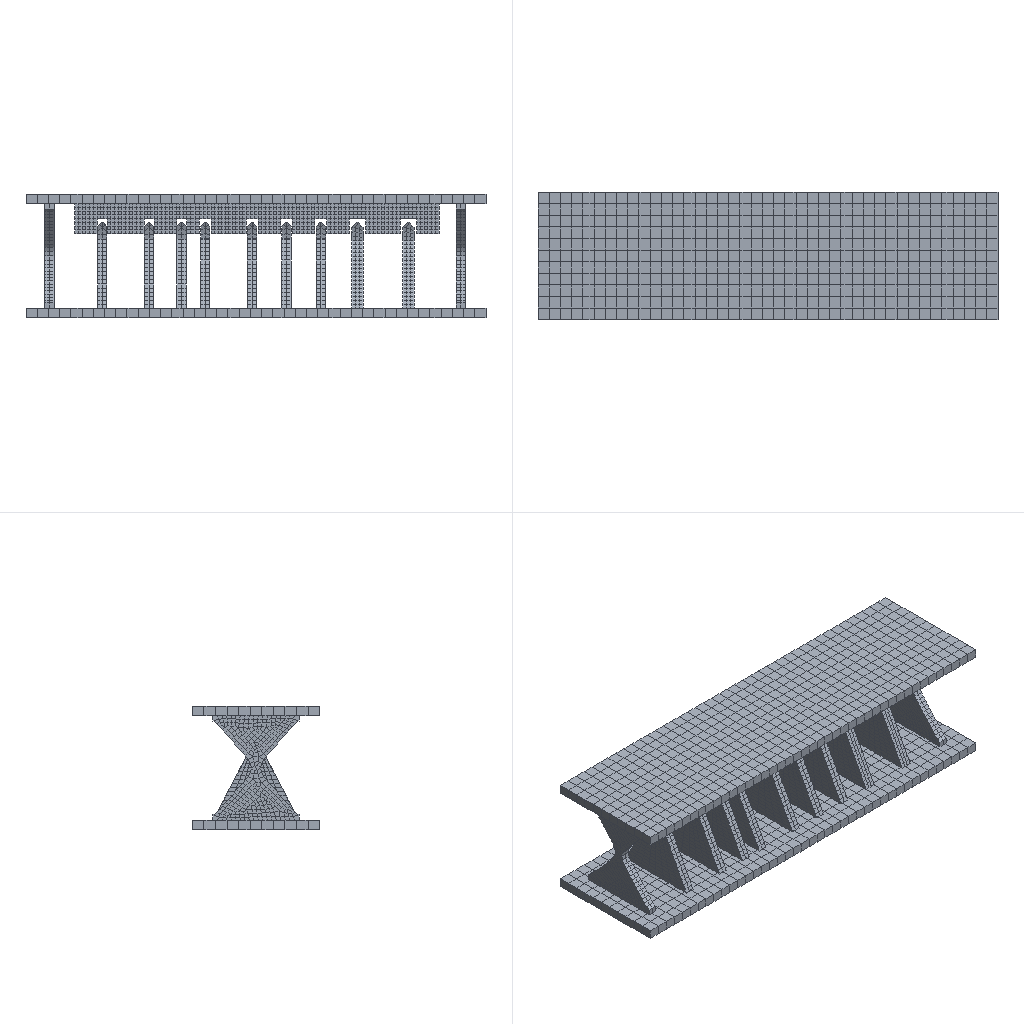Simulation study | abaqus
Abaqus input file, long lists of numbers shortened:
*Heading
** Job name: deck-2 Model name: 0815
** Generated by: Abaqus/CAE 2024
*Preprint, echo=NO, model=NO, history=NO, contact=NO
**
** PARTS
**
*Part, name=Part-1
*Node
      1,      1227.62,         340.,          25.
      2,      1227.62,   309.091,          25.
** (1006 more lines like these left out)
*Element, type=C3D8R
  1,   25,   26,   38,   37,    1,    2,   14,   13
  2,   26,   27,   39,   38,    2,    3,   15,   14
** (449 more lines like these left out)
*Nset, nset=_PickedSet5, internal, generate
    1,  1008,     1
*Elset, elset=_PickedSet5, internal, generate
   1,  451,    1
** Section: q235
*Solid Section, elset=_PickedSet5, controls=EC-1, material=q235
,
*End Part
**
*Part, name=Part-7
*Node
      1,   51318.848,   20056.129,           0.
      2,      51308.5,   20050.193,           0.
** (1084 more lines like these left out)
*Element, type=C3D8R
  1,  119,    1,    2,  145,  481,  363,  364,  507
  2,    1,  119,  116,   23,  363,  481,  478,  385
** (622 more lines like these left out)
*Nset, nset=Set-1, generate
    1,  1086,     1
*Elset, elset=Set-1, generate
   1,  624,    1
** Section: Section-2
*Solid Section, elset=Set-1, material=q235
,
*End Part
**
*Part, name=Part-8
*Node
      1,   44.972,         218.,           0.
      2,   50.449,         230.,          10.
** (601 more lines like these left out)
*Element, type=C3D8R
 1, 164,  20, 157, 481,  18,   1,  19, 155
 2, 165,  21, 158, 480, 164,  20, 157, 481
** (334 more lines like these left out)
*Nset, nset=Set-1, generate
   1,  603,    1
*Elset, elset=Set-1, generate
   1,  336,    1
** Section: Section-2
*Solid Section, elset=Set-1, material=q235
,
*End Part
**
*Part, name=Part-9
*Node
      1,  -916.483,   84.154,           0.
      2,  -916.483,   84.154,          40.
** (4008 more lines like these left out)
*Element, type=C3D8R
 1,  158, 1029, 2787,  999,    1,  121,  969,  136
 2, 1029, 1030, 2788, 2787,  121,  122,  970,  969
** (2638 more lines like these left out)
*Nset, nset=Set-1, generate
    1,  4010,     1
*Elset, elset=Set-1, generate
    1,  2640,     1
** Section: Section-2
*Solid Section, elset=Set-1, material=q235
,
*End Part
**
*Part, name=Part-10
*Node
      1,   4.129,   256.243,          25.
      2,   4.785,   252.357,          25.
** (558 more lines like these left out)
*Element, type=C3D8R
 1,  36,  43, 171, 165,   1,   2,  21,  22
 2, 165, 171,  42,  25,  22,  21,   3,   4
** (306 more lines like these left out)
*Nset, nset=Set-1
   1,   2,   3,   4,   5,   6,   7,   8,  17,  18,  19,  20,  21,  22,  23,  24
  25,  26,  27,  28,  29,  30,  31,  32,  33,  34,  35,  36,  37,  38,  39,  40
** (27 more lines like these left out)
*Elset, elset=Set-1
   1,   2,   3,   4,   5,   6,   7,   8,   9,  10,  11,  12,  13,  14,  71,  72
  73,  74,  75,  76,  77,  78,  79,  80,  81,  82,  83,  84,  85,  86,  87,  88
** (14 more lines like these left out)
*Nset, nset=_PickedSet10, internal, generate
   1,  560,    1
*Elset, elset=_PickedSet10, internal, generate
   1,  308,    1
** Section: Section-2
*Solid Section, elset=_PickedSet10, material=q235
,
*End Part
**
*Part, name=Part-11
*Node
      1,  -175.665,   409.503,         17.5
      2,  -105.665,   409.503,         17.5
** (878 more lines like these left out)
*Element, type=C3D8R
  1,   4,  22,   7,   1,  44,  62,  47,  41
  2,  22,  21,   8,   7,  62,  61,  48,  47
** (565 more lines like these left out)
*Nset, nset=Set-1, generate
   1,  880,    1
*Elset, elset=Set-1, generate
   1,  567,    1
** Section: Section-2
*Solid Section, elset=Set-1, material=q235
,
*End Part
**
**
** ASSEMBLY
**
*Assembly, name=Assembly
**
*Instance, name=Part-1-1, part=Part-1
*End Instance
**
*Instance, name=Part-1-1-lin-2-1, part=Part-1
          0.,           0.,         305.
*End Instance
**
*Instance, name=Part-7-1, part=Part-7
50.,     -51253.5, -20010.046
50.,     -51253.5, -20010.046, 50.577, -51252.923, -20009.469,         120.
*End Instance
**
*Instance, name=Part-7-1-lin-2-1, part=Part-7
     1147.62,     -51253.5, -20010.046
     1147.62,     -51253.5, -20010.046, 1148.197, -51252.923, -20009.469,         120.
*End Instance
**
*Instance, name=Part-9-1, part=Part-9
 1106.483,         190.,   180.846
 1106.483,         190.,   180.846, 1107.483,         190.,   180.846, 90.
*End Instance
**
*Instance, name=Part-8-1, part=Part-8
      190.85,   152.051,          25.
      190.85,   152.051,          25., 191.427, 152.628, 25.577,         120.
*End Instance
**
*Instance, name=Part-8-1-lin-1-2, part=Part-8
      315.85,   152.051,          25.
      315.85,   152.051,          25., 316.427, 152.628, 25.577,         120.
*End Instance
**
*Instance, name=Part-8-1-lin-1-2-lin-2-1, part=Part-8
      402.55,   152.051,          25.
      402.55,   152.051,          25., 403.127, 152.628, 25.577,         120.
*End Instance
**
*Instance, name=Part-10-1, part=Part-10
      465.85,   184.157,    -44.124
      465.85,   184.157,    -44.124, 466.427, 184.734, -43.547,         120.
*End Instance
**
*Instance, name=Part-10-1-lin-2-1, part=Part-10
      590.85,   184.157,    -44.124
      590.85,   184.157,    -44.124, 591.427, 184.734, -43.547,         120.
*End Instance
**
*Instance, name=Part-10-1-lin-3-1, part=Part-10
      774.37,   184.157,    -44.124
      774.37,   184.157,    -44.124, 774.947, 184.734, -43.547,         120.
*End Instance
**
*Instance, name=Part-10-1-lin-4-1, part=Part-10
      682.61,   184.157,    -44.124
      682.61,   184.157,    -44.124, 683.187, 184.734, -43.547,         120.
*End Instance
**
*Instance, name=Part-11-1, part=Part-11
      869.52,   310.665,   -154.503
      869.52,   310.665,   -154.503, 870.097, 311.242, -153.925,         120.
*End Instance
**
*Instance, name=Part-11-1-lin-2-1, part=Part-11
     1005.85,   310.665,   -154.503
     1005.85,   310.665,   -154.503, 1006.427, 311.242, -153.925,         120.
*End Instance
**
*Node
      1,   613.81,         170.,         500.
*Node
      2,   613.81,         170.,        -200.
*Nset, nset=Set-1, instance=Part-1-1
   13,   14,   15,   16,   17,   18,   19,   20,   21,   22,   23,   24,   37,   38,   39,   40
   41,   42,   43,   44,   45,   46,   47,   48,   61,   62,   63,   64,   65,   66,   67,   68
** (30 more lines like these left out)
*Elset, elset=Set-1, instance=Part-1-1, generate
   1,  451,    1
*Nset, nset=Set-6
 2,
*Nset, nset=Set-7
 1,
*Nset, nset=m_Set-5
 2,
*Nset, nset=rp1
 1,
*Nset, nset=rp2
 2,
*Nset, nset=_PickedSet71, internal
 1,
*Nset, nset=_PickedSet120, internal
 1,
*Nset, nset=_PickedSet121, internal
 2,
*Elset, elset=_m_Surf-12_S5, internal, instance=Part-1-1-lin-2-1, generate
   1,  451,    1
*Surface, type=ELEMENT, name=m_Surf-12
_m_Surf-12_S5, S5
*Elset, elset=_m_Surf-13_S3, internal, instance=Part-1-1, generate
   1,  451,    1
*Surface, type=ELEMENT, name=m_Surf-13
_m_Surf-13_S3, S3
*Elset, elset=_m_Surf-17_S3, internal, instance=Part-1-1, generate
   1,  451,    1
*Surface, type=ELEMENT, name=m_Surf-17
_m_Surf-17_S3, S3
*Elset, elset=_m_Surf-19_S5, internal, instance=Part-1-1-lin-2-1, generate
   1,  451,    1
*Surface, type=ELEMENT, name=m_Surf-19
_m_Surf-19_S5, S5
*Elset, elset=_m_Surf-28_S5, internal, instance=Part-8-1
  82,  83,  84,  85,  86,  87,  88,  89,  90,  91,  92,  93,  94,  95,  96,  97
  98, 116, 117, 118, 119, 120, 121, 122, 123, 124, 125, 126, 127, 128, 129, 130
** (7 more lines like these left out)
*Elset, elset=_m_Surf-28_S5, internal, instance=Part-8-1-lin-1-2
  82,  83,  84,  85,  86,  87,  88,  89,  90,  91,  92,  93,  94,  95,  96,  97
  98, 116, 117, 118, 119, 120, 121, 122, 123, 124, 125, 126, 127, 128, 129, 130
** (7 more lines like these left out)
*Elset, elset=_m_Surf-28_S5, internal, instance=Part-8-1-lin-1-2-lin-2-1
  82,  83,  84,  85,  86,  87,  88,  89,  90,  91,  92,  93,  94,  95,  96,  97
  98, 116, 117, 118, 119, 120, 121, 122, 123, 124, 125, 126, 127, 128, 129, 130
** (7 more lines like these left out)
*Elset, elset=_m_Surf-28_S5, internal, instance=Part-10-1-lin-2-1, generate
  2,  14,   2
*Elset, elset=_m_Surf-28_S5, internal, instance=Part-10-1-lin-4-1, generate
  2,  14,   2
*Elset, elset=_m_Surf-28_S5, internal, instance=Part-10-1, generate
  2,  14,   2
*Elset, elset=_m_Surf-28_S5, internal, instance=Part-10-1-lin-3-1, generate
  2,  14,   2
*Elset, elset=_m_Surf-28_S3, internal, instance=Part-8-1
  65,  66,  67,  68,  69,  70,  71,  72,  73,  74,  75,  76,  77,  78,  79,  80
  81,  99, 100, 101, 102, 103, 104, 105, 106, 107, 108, 109, 110, 111, 112, 113
** (7 more lines like these left out)
*Elset, elset=_m_Surf-28_S3, internal, instance=Part-8-1-lin-1-2
  65,  66,  67,  68,  69,  70,  71,  72,  73,  74,  75,  76,  77,  78,  79,  80
  81,  99, 100, 101, 102, 103, 104, 105, 106, 107, 108, 109, 110, 111, 112, 113
** (7 more lines like these left out)
*Elset, elset=_m_Surf-28_S3, internal, instance=Part-8-1-lin-1-2-lin-2-1
  65,  66,  67,  68,  69,  70,  71,  72,  73,  74,  75,  76,  77,  78,  79,  80
  81,  99, 100, 101, 102, 103, 104, 105, 106, 107, 108, 109, 110, 111, 112, 113
** (7 more lines like these left out)
*Elset, elset=_m_Surf-28_S3, internal, instance=Part-10-1-lin-2-1, generate
  1,  13,   2
*Elset, elset=_m_Surf-28_S3, internal, instance=Part-10-1-lin-4-1, generate
  1,  13,   2
*Elset, elset=_m_Surf-28_S3, internal, instance=Part-10-1, generate
  1,  13,   2
*Elset, elset=_m_Surf-28_S3, internal, instance=Part-10-1-lin-3-1, generate
  1,  13,   2
*Elset, elset=_m_Surf-28_S4, internal, instance=Part-10-1-lin-2-1, generate
  72,  308,    2
*Elset, elset=_m_Surf-28_S4, internal, instance=Part-10-1-lin-4-1, generate
  72,  308,    2
*Elset, elset=_m_Surf-28_S4, internal, instance=Part-10-1, generate
  72,  308,    2
*Elset, elset=_m_Surf-28_S4, internal, instance=Part-10-1-lin-3-1, generate
  72,  308,    2
*Elset, elset=_m_Surf-28_S6, internal, instance=Part-10-1-lin-2-1, generate
  71,  307,    2
*Elset, elset=_m_Surf-28_S6, internal, instance=Part-10-1-lin-4-1, generate
  71,  307,    2
*Elset, elset=_m_Surf-28_S6, internal, instance=Part-10-1, generate
  71,  307,    2
*Elset, elset=_m_Surf-28_S6, internal, instance=Part-10-1-lin-3-1, generate
  71,  307,    2
*Elset, elset=_m_Surf-28_S1, internal, instance=Part-10-1-lin-2-1
 13, 14
*Elset, elset=_m_Surf-28_S1, internal, instance=Part-10-1-lin-4-1
 13, 14
*Elset, elset=_m_Surf-28_S1, internal, instance=Part-10-1
 13, 14
*Elset, elset=_m_Surf-28_S1, internal, instance=Part-10-1-lin-3-1
 13, 14
*Elset, elset=_m_Surf-28_S2, internal, instance=Part-10-1-lin-2-1
 1, 2
*Elset, elset=_m_Surf-28_S2, internal, instance=Part-10-1-lin-4-1
 1, 2
*Elset, elset=_m_Surf-28_S2, internal, instance=Part-10-1
 1, 2
*Elset, elset=_m_Surf-28_S2, internal, instance=Part-10-1-lin-3-1
 1, 2
*Surface, type=ELEMENT, name=m_Surf-28
_m_Surf-28_S5, S5
_m_Surf-28_S3, S3
_m_Surf-28_S4, S4
_m_Surf-28_S6, S6
_m_Surf-28_S2, S2
_m_Surf-28_S1, S1
*Elset, elset=_m_Surf-30_S4, internal, instance=Part-8-1
  1,  2,  3,  4,  5,  6,  7,  8,  9, 10, 11, 12, 13, 14, 15, 16
 25, 26, 27, 28, 29, 30, 31, 32, 36, 37, 38, 39, 40, 44, 48, 52
** (1 more lines like these left out)
*Elset, elset=_m_Surf-30_S4, internal, instance=Part-8-1-lin-1-2
  1,  2,  3,  4,  5,  6,  7,  8,  9, 10, 11, 12, 13, 14, 15, 16
 25, 26, 27, 28, 29, 30, 31, 32, 36, 37, 38, 39, 40, 44, 48, 52
** (1 more lines like these left out)
*Elset, elset=_m_Surf-30_S4, internal, instance=Part-8-1-lin-1-2-lin-2-1
  1,  2,  3,  4,  5,  6,  7,  8,  9, 10, 11, 12, 13, 14, 15, 16
 25, 26, 27, 28, 29, 30, 31, 32, 36, 37, 38, 39, 40, 44, 48, 52
** (1 more lines like these left out)
*Elset, elset=_m_Surf-30_S4, internal, instance=Part-10-1-lin-2-1
  15,  16,  17,  18,  19,  20,  21,  22,  23,  24,  25,  26,  33,  34,  35,  36
  37,  38,  42,  43,  44,  45,  46,  50,  54,  58,  62,  66,  70,  72,  74,  76
** (8 more lines like these left out)
*Elset, elset=_m_Surf-30_S4, internal, instance=Part-10-1-lin-4-1
  15,  16,  17,  18,  19,  20,  21,  22,  23,  24,  25,  26,  33,  34,  35,  36
  37,  38,  42,  43,  44,  45,  46,  50,  54,  58,  62,  66,  70,  72,  74,  76
** (8 more lines like these left out)
*Elset, elset=_m_Surf-30_S4, internal, instance=Part-11-1-lin-2-1, generate
   9,  549,   27
*Elset, elset=_m_Surf-30_S4, internal, instance=Part-10-1
  15,  16,  17,  18,  19,  20,  21,  22,  23,  24,  25,  26,  33,  34,  35,  36
  37,  38,  42,  43,  44,  45,  46,  50,  54,  58,  62,  66,  70,  72,  74,  76
** (8 more lines like these left out)
*Elset, elset=_m_Surf-30_S4, internal, instance=Part-11-1, generate
   9,  549,   27
*Elset, elset=_m_Surf-30_S4, internal, instance=Part-10-1-lin-3-1
  15,  16,  17,  18,  19,  20,  21,  22,  23,  24,  25,  26,  33,  34,  35,  36
  37,  38,  42,  43,  44,  45,  46,  50,  54,  58,  62,  66,  70,  72,  74,  76
** (8 more lines like these left out)
*Elset, elset=_m_Surf-30_S3, internal, instance=Part-8-1
   1,   2,   3,   4,   5,   6,   7,   8,   9,  10,  11,  12,  13,  14,  15,  16
  17,  18,  19,  20,  21,  22,  23,  24,  33,  34,  35,  36,  37,  49,  50,  51
** (10 more lines like these left out)
*Elset, elset=_m_Surf-30_S3, internal, instance=Part-8-1-lin-1-2
   1,   2,   3,   4,   5,   6,   7,   8,   9,  10,  11,  12,  13,  14,  15,  16
  17,  18,  19,  20,  21,  22,  23,  24,  33,  34,  35,  36,  37,  49,  50,  51
** (10 more lines like these left out)
*Elset, elset=_m_Surf-30_S3, internal, instance=Part-8-1-lin-1-2-lin-2-1
   1,   2,   3,   4,   5,   6,   7,   8,   9,  10,  11,  12,  13,  14,  15,  16
  17,  18,  19,  20,  21,  22,  23,  24,  33,  34,  35,  36,  37,  49,  50,  51
** (10 more lines like these left out)
*Elset, elset=_m_Surf-30_S3, internal, instance=Part-10-1-lin-2-1
   1,   3,   5,   7,   9,  11,  13,  15,  16,  17,  18,  19,  20,  21,  22,  23
  24,  25,  26,  27,  28,  29,  30,  31,  32,  39,  40,  41,  42,  43,  55,  56
** (3 more lines like these left out)
*Elset, elset=_m_Surf-30_S3, internal, instance=Part-10-1-lin-4-1
   1,   3,   5,   7,   9,  11,  13,  15,  16,  17,  18,  19,  20,  21,  22,  23
  24,  25,  26,  27,  28,  29,  30,  31,  32,  39,  40,  41,  42,  43,  55,  56
** (3 more lines like these left out)
*Elset, elset=_m_Surf-30_S3, internal, instance=Part-11-1-lin-2-1
   1,   2,   3,   4,   5,   6,   7,   8,   9,  26,  27,  28,  29,  30,  31,  32
  33,  34,  35,  36,  53,  54,  55,  56,  57,  58,  59,  60,  61,  62,  63,  80
** (13 more lines like these left out)
*Elset, elset=_m_Surf-30_S3, internal, instance=Part-10-1
   1,   3,   5,   7,   9,  11,  13,  15,  16,  17,  18,  19,  20,  21,  22,  23
  24,  25,  26,  27,  28,  29,  30,  31,  32,  39,  40,  41,  42,  43,  55,  56
** (3 more lines like these left out)
*Elset, elset=_m_Surf-30_S3, internal, instance=Part-11-1
   1,   2,   3,   4,   5,   6,   7,   8,   9,  26,  27,  28,  29,  30,  31,  32
  33,  34,  35,  36,  53,  54,  55,  56,  57,  58,  59,  60,  61,  62,  63,  80
** (13 more lines like these left out)
*Elset, elset=_m_Surf-30_S3, internal, instance=Part-10-1-lin-3-1
   1,   3,   5,   7,   9,  11,  13,  15,  16,  17,  18,  19,  20,  21,  22,  23
  24,  25,  26,  27,  28,  29,  30,  31,  32,  39,  40,  41,  42,  43,  55,  56
** (3 more lines like these left out)
*Elset, elset=_m_Surf-30_S2, internal, instance=Part-8-1
  1,  5,  9, 13, 17, 18, 25, 26, 33, 34, 35, 36, 37, 38, 39, 40
 41, 42, 43, 44, 45, 46, 47, 48, 57, 61, 65, 66, 67, 68, 69, 70
** (2 more lines like these left out)
*Elset, elset=_m_Surf-30_S2, internal, instance=Part-8-1-lin-1-2
  1,  5,  9, 13, 17, 18, 25, 26, 33, 34, 35, 36, 37, 38, 39, 40
 41, 42, 43, 44, 45, 46, 47, 48, 57, 61, 65, 66, 67, 68, 69, 70
** (2 more lines like these left out)
*Elset, elset=_m_Surf-30_S2, internal, instance=Part-8-1-lin-1-2-lin-2-1
  1,  5,  9, 13, 17, 18, 25, 26, 33, 34, 35, 36, 37, 38, 39, 40
 41, 42, 43, 44, 45, 46, 47, 48, 57, 61, 65, 66, 67, 68, 69, 70
** (2 more lines like these left out)
*Elset, elset=_m_Surf-30_S2, internal, instance=Part-10-1-lin-2-1
  1,  2, 15, 18, 21, 24, 27, 28, 33, 34, 39, 40, 41, 42, 43, 44
 45, 46, 47, 48, 49, 50, 51, 52, 53, 54, 63, 64, 65, 66, 67, 68
** (1 more lines like these left out)
*Elset, elset=_m_Surf-30_S2, internal, instance=Part-10-1-lin-4-1
  1,  2, 15, 18, 21, 24, 27, 28, 33, 34, 39, 40, 41, 42, 43, 44
 45, 46, 47, 48, 49, 50, 51, 52, 53, 54, 63, 64, 65, 66, 67, 68
** (1 more lines like these left out)
*Elset, elset=_m_Surf-30_S2, internal, instance=Part-10-1
  1,  2, 15, 18, 21, 24, 27, 28, 33, 34, 39, 40, 41, 42, 43, 44
 45, 46, 47, 48, 49, 50, 51, 52, 53, 54, 63, 64, 65, 66, 67, 68
** (1 more lines like these left out)
*Elset, elset=_m_Surf-30_S2, internal, instance=Part-10-1-lin-3-1
  1,  2, 15, 18, 21, 24, 27, 28, 33, 34, 39, 40, 41, 42, 43, 44
 45, 46, 47, 48, 49, 50, 51, 52, 53, 54, 63, 64, 65, 66, 67, 68
** (1 more lines like these left out)
*Elset, elset=_m_Surf-30_S5, internal, instance=Part-8-1
  82,  83,  84,  85,  86,  87,  88,  89,  90,  91,  92,  93,  94,  95,  96,  97
  98, 116, 117, 118, 119, 120, 121, 122, 123, 124, 125, 126, 127, 128, 129, 130
** (7 more lines like these left out)
*Elset, elset=_m_Surf-30_S5, internal, instance=Part-8-1-lin-1-2
  82,  83,  84,  85,  86,  87,  88,  89,  90,  91,  92,  93,  94,  95,  96,  97
  98, 116, 117, 118, 119, 120, 121, 122, 123, 124, 125, 126, 127, 128, 129, 130
** (7 more lines like these left out)
*Elset, elset=_m_Surf-30_S5, internal, instance=Part-8-1-lin-1-2-lin-2-1
  82,  83,  84,  85,  86,  87,  88,  89,  90,  91,  92,  93,  94,  95,  96,  97
  98, 116, 117, 118, 119, 120, 121, 122, 123, 124, 125, 126, 127, 128, 129, 130
** (7 more lines like these left out)
*Elset, elset=_m_Surf-30_S5, internal, instance=Part-10-1-lin-2-1
   2,   4,   6,   8,  10,  12,  14,  83,  84,  97,  98, 111, 112, 125, 126, 139
 140, 153, 154, 167, 168, 181, 182, 195, 196, 209, 210, 223, 224, 237, 238, 251
** (1 more lines like these left out)
*Elset, elset=_m_Surf-30_S5, internal, instance=Part-10-1-lin-4-1
   2,   4,   6,   8,  10,  12,  14,  83,  84,  97,  98, 111, 112, 125, 126, 139
 140, 153, 154, 167, 168, 181, 182, 195, 196, 209, 210, 223, 224, 237, 238, 251
** (1 more lines like these left out)
*Elset, elset=_m_Surf-30_S5, internal, instance=Part-11-1-lin-2-1
  10,  11,  37,  38,  64,  65,  91,  92, 118, 119, 145, 146, 172, 173, 199, 200
 226, 227, 253, 254, 280, 281, 307, 308, 334, 335, 361, 362, 388, 389, 415, 416
** (1 more lines like these left out)
*Elset, elset=_m_Surf-30_S5, internal, instance=Part-10-1
   2,   4,   6,   8,  10,  12,  14,  83,  84,  97,  98, 111, 112, 125, 126, 139
 140, 153, 154, 167, 168, 181, 182, 195, 196, 209, 210, 223, 224, 237, 238, 251
** (1 more lines like these left out)
*Elset, elset=_m_Surf-30_S5, internal, instance=Part-11-1
  10,  11,  37,  38,  64,  65,  91,  92, 118, 119, 145, 146, 172, 173, 199, 200
 226, 227, 253, 254, 280, 281, 307, 308, 334, 335, 361, 362, 388, 389, 415, 416
** (1 more lines like these left out)
*Elset, elset=_m_Surf-30_S5, internal, instance=Part-10-1-lin-3-1
   2,   4,   6,   8,  10,  12,  14,  83,  84,  97,  98, 111, 112, 125, 126, 139
 140, 153, 154, 167, 168, 181, 182, 195, 196, 209, 210, 223, 224, 237, 238, 251
** (1 more lines like these left out)
*Elset, elset=_m_Surf-30_S1, internal, instance=Part-8-1, generate
 303,  336,    1
*Elset, elset=_m_Surf-30_S1, internal, instance=Part-8-1-lin-1-2, generate
 303,  336,    1
*Elset, elset=_m_Surf-30_S1, internal, instance=Part-8-1-lin-1-2-lin-2-1, generate
 303,  336,    1
*Elset, elset=_m_Surf-30_S1, internal, instance=Part-10-1-lin-2-1
 13, 14
*Elset, elset=_m_Surf-30_S1, internal, instance=Part-10-1-lin-4-1
 13, 14
*Elset, elset=_m_Surf-30_S1, internal, instance=Part-11-1-lin-2-1, generate
  1,  27,   1
*Elset, elset=_m_Surf-30_S1, internal, instance=Part-10-1
 13, 14
*Elset, elset=_m_Surf-30_S1, internal, instance=Part-11-1, generate
  1,  27,   1
*Elset, elset=_m_Surf-30_S1, internal, instance=Part-10-1-lin-3-1
 13, 14
*Elset, elset=_m_Surf-30_S6, internal, instance=Part-10-1-lin-2-1, generate
  71,  307,    2
*Elset, elset=_m_Surf-30_S6, internal, instance=Part-10-1-lin-4-1, generate
  71,  307,    2
*Elset, elset=_m_Surf-30_S6, internal, instance=Part-11-1-lin-2-1
   1,  10,  12,  14,  16,  18,  20,  22,  24,  26,  28,  37,  39,  41,  43,  45
  47,  49,  51,  53,  55,  64,  66,  68,  70,  72,  74,  76,  78,  80,  82,  91
** (12 more lines like these left out)
*Elset, elset=_m_Surf-30_S6, internal, instance=Part-10-1, generate
  71,  307,    2
*Elset, elset=_m_Surf-30_S6, internal, instance=Part-11-1
   1,  10,  12,  14,  16,  18,  20,  22,  24,  26,  28,  37,  39,  41,  43,  45
  47,  49,  51,  53,  55,  64,  66,  68,  70,  72,  74,  76,  78,  80,  82,  91
** (12 more lines like these left out)
*Elset, elset=_m_Surf-30_S6, internal, instance=Part-10-1-lin-3-1, generate
  71,  307,    2
*Surface, type=ELEMENT, name=m_Surf-30
_m_Surf-30_S4, S4
_m_Surf-30_S3, S3
_m_Surf-30_S2, S2
_m_Surf-30_S6, S6
_m_Surf-30_S5, S5
_m_Surf-30_S1, S1
*Elset, elset=_s_Surf-1_S3, internal, instance=Part-1-1, generate
   1,  451,    1
*Surface, type=ELEMENT, name=s_Surf-1
_s_Surf-1_S3, S3
*Elset, elset=_s_Surf-3_S5, internal, instance=Part-1-1-lin-2-1, generate
   1,  451,    1
*Surface, type=ELEMENT, name=s_Surf-3
_s_Surf-3_S5, S5
*Elset, elset=_s_Surf-14_S4, internal, instance=Part-1-1, generate
  11,  451,   11
*Surface, type=ELEMENT, name=s_Surf-14
_s_Surf-14_S4, S4
*Elset, elset=_s_Surf-17_S5, internal, instance=Part-1-1, generate
   1,  451,    1
*Surface, type=ELEMENT, name=s_Surf-17
_s_Surf-17_S5, S5
*Elset, elset=_s_Surf-26_S4, internal, instance=Part-7-1
  15, 327
*Elset, elset=_s_Surf-26_S4, internal, instance=Part-7-1-lin-2-1
  15, 327
*Elset, elset=_s_Surf-26_S4, internal, instance=Part-9-1
 2036, 2040, 2044, 2048, 2052, 2056, 2060, 2064, 2068, 2072, 2076, 2080, 2132, 2136, 2140, 2144
 2148, 2152, 2156, 2160, 2164, 2168, 2172, 2176, 2372, 2376, 2380, 2384, 2388, 2392, 2396, 2400
** (1 more lines like these left out)
*Elset, elset=_s_Surf-26_S5, internal, instance=Part-7-1
  16,  33,  42, 111, 124, 133, 135, 138, 328, 345, 354, 423, 436, 445, 447, 450
*Elset, elset=_s_Surf-26_S5, internal, instance=Part-7-1-lin-2-1
  16,  33,  42, 111, 124, 133, 135, 138, 328, 345, 354, 423, 436, 445, 447, 450
*Elset, elset=_s_Surf-26_S3, internal, instance=Part-7-1
  35,  37,  39,  48, 114, 115, 116, 118, 119, 143, 347, 349, 351, 360, 426, 427
 428, 430, 431, 455
*Elset, elset=_s_Surf-26_S3, internal, instance=Part-7-1-lin-2-1
  35,  37,  39,  48, 114, 115, 116, 118, 119, 143, 347, 349, 351, 360, 426, 427
 428, 430, 431, 455
*Elset, elset=_s_Surf-26_S1, internal, instance=Part-9-1
   73,   74,   75,   76,   77,   78,   79,   80,   81,   82,   83,   84,   85,   86,   87,   88
   89,   90,   91,   92,   93,   94,   95,   96,  217,  218,  219,  220,  221,  222,  223,  224
** (18 more lines like these left out)
*Elset, elset=_s_Surf-26_S2, internal, instance=Part-9-1, generate
 2497,  2532,     1
*Surface, type=ELEMENT, name=s_Surf-26
_s_Surf-26_S4, S4
_s_Surf-26_S5, S5
_s_Surf-26_S2, S2
_s_Surf-26_S3, S3
_s_Surf-26_S1, S1
*Elset, elset=_s_Surf-27_S5, internal, instance=Part-7-1
  20,  22,  62,  79,  87,  90,  95,  97, 154, 332, 334, 374, 391, 399, 402, 407
 409, 466
*Elset, elset=_s_Surf-27_S5, internal, instance=Part-7-1-lin-2-1
  20,  22,  62,  79,  87,  90,  95,  97, 154, 332, 334, 374, 391, 399, 402, 407
 409, 466
*Elset, elset=_s_Surf-27_S3, internal, instance=Part-7-1
  69,  76,  77,  81,  85,  86,  89,  98, 106, 381, 388, 389, 393, 397, 398, 401
 410, 418
*Elset, elset=_s_Surf-27_S3, internal, instance=Part-7-1-lin-2-1
  69,  76,  77,  81,  85,  86,  89,  98, 106, 381, 388, 389, 393, 397, 398, 401
 410, 418
*Elset, elset=_s_Surf-27_S6, internal, instance=Part-7-1
  72, 384
*Elset, elset=_s_Surf-27_S6, internal, instance=Part-7-1-lin-2-1
  72, 384
*Elset, elset=_s_Surf-27_S4, internal, instance=Part-8-1-lin-1-2, generate
  81,  336,   17
*Elset, elset=_s_Surf-27_S4, internal, instance=Part-8-1, generate
  81,  336,   17
*Elset, elset=_s_Surf-27_S4, internal, instance=Part-8-1-lin-1-2-lin-2-1, generate
  81,  336,   17
*Elset, elset=_s_Surf-27_S2, internal, instance=Part-10-1-lin-4-1, generate
 295,  308,    1
*Elset, elset=_s_Surf-27_S2, internal, instance=Part-10-1-lin-2-1, generate
 295,  308,    1
*Elset, elset=_s_Surf-27_S2, internal, instance=Part-11-1-lin-2-1, generate
 541,  567,    1
*Elset, elset=_s_Surf-27_S2, internal, instance=Part-10-1, generate
 295,  308,    1
*Elset, elset=_s_Surf-27_S2, internal, instance=Part-11-1, generate
 541,  567,    1
*Elset, elset=_s_Surf-27_S2, internal, instance=Part-10-1-lin-3-1, generate
 295,  308,    1
*Surface, type=ELEMENT, name=s_Surf-27
_s_Surf-27_S5, S5
_s_Surf-27_S3, S3
_s_Surf-27_S6, S6
_s_Surf-27_S4, S4
_s_Surf-27_S2, S2
*Elset, elset=_s_Surf-28_S5, internal, instance=Part-9-1
   21,   22,   23,   24,   45,   46,   47,   48,   69,   70,   71,   72,   93,   94,   95,   96
  869,  870,  871,  872,  893,  894,  895,  896,  917,  918,  919,  920,  941,  942,  943,  944
** (19 more lines like these left out)
*Elset, elset=_s_Surf-28_S4, internal, instance=Part-9-1
    4,    8,   12,   16,   20,   24,   28,   32,   36,   40,   44,   48,   52,   56,   60,   64
   68,   72,   76,   80,   84,   88,   92,   96,  100,  104,  108,  112,  116,  120,  124,  128
** (30 more lines like these left out)
*Elset, elset=_s_Surf-28_S6, internal, instance=Part-9-1
    1,    5,    9,   13,   17,   21,   25,   29,   33,   37,   41,   45,   49,   53,   57,   61
   65,   69,   73,   77,   81,   85,   89,   93,   97,  101,  105,  109,  113,  117,  121,  125
** (35 more lines like these left out)
*Elset, elset=_s_Surf-28_S3, internal, instance=Part-9-1
  945,  946,  947,  948,  969,  970,  971,  972,  993,  994,  995,  996, 1017, 1018, 1019, 1020
 1041, 1042, 1043, 1044, 1081, 1082, 1083, 1084, 1121, 1122, 1123, 1124, 1161, 1162, 1163, 1164
** (17 more lines like these left out)
*Elset, elset=_s_Surf-28_S2, internal, instance=Part-9-1
 1017, 1018, 1019, 1020, 1021, 1022, 1023, 1024, 1025, 1026, 1027, 1028, 1029, 1030, 1031, 1032
 1033, 1034, 1035, 1036, 1037, 1038, 1039, 1040, 1161, 1162, 1163, 1164, 1165, 1166, 1167, 1168
** (19 more lines like these left out)
*Elset, elset=_s_Surf-28_S1, internal, instance=Part-9-1, generate
 2017,  2032,     1
*Surface, type=ELEMENT, name=s_Surf-28
_s_Surf-28_S5, S5
_s_Surf-28_S4, S4
_s_Surf-28_S6, S6
_s_Surf-28_S2, S2
_s_Surf-28_S3, S3
_s_Surf-28_S1, S1
*Elset, elset=__PickedSurf70_S3, internal, instance=Part-1-1-lin-2-1, generate
   1,  451,    1
*Surface, type=ELEMENT, name=_PickedSurf70, internal
__PickedSurf70_S3, S3
** Constraint: Constraint-2
*Tie, name=Constraint-2, adjust=yes
s_Surf-26, m_Surf-12
** Constraint: Constraint-3
*Tie, name=Constraint-3, adjust=yes
s_Surf-27, m_Surf-13
** Constraint: Constraint-4
*Coupling, constraint name=Constraint-4, ref node=m_Set-5, surface=s_Surf-17
*Kinematic
** Constraint: rp-1
*Coupling, constraint name=rp-1, ref node=_PickedSet71, surface=_PickedSurf70
*Kinematic
*End Assembly
**
** ELEMENT CONTROLS
**
*Section Controls, name=EC-1, VISCOSITY=0.0001
1., 1., 1.
*Amplitude, name=Amp-1
             0.,              0.,              1.,              5.,              2.,              0.,              3.,             -5.
             4.,              0.,              5.,              5.,              6.,              0.,              7.,             -5.
             8.,              0.,              9.,              5.,             10.,              0.,             11.,             -5.
            12.,              0.,             13.,             10.,             14.,              0.,             15.,            -10.
            16.,              0.,             17.,             10.,             18.,              0.,             19.,            -10.
            20.,              0.,             21.,             10.,             22.,              0.,             23.,            -10.
            24.,              0.,             25.,             15.,             26.,              0.,             27.,            -15.
            28.,              0.,             29.,             15.,             30.,              0.,             31.,            -15.
            32.,              0.,             33.,             15.,             34.,              0.,             35.,            -15.
            36.,              0.,             37.,             20.,             38.,              0.,             39.,            -20.
            40.,              0.,             41.,             20.,             42.,              0.,             43.,            -20.
            44.,              0.,             45.,             20.,             46.,              0.,             47.,            -20.
            48.,              0.,             49.,             25.,             50.,              0.,             51.,            -25.
            52.,              0.,             53.,             25.,             54.,              0.,             55.,            -25.
            56.,              0.,             57.,             25.,             58.,              0.,             59.,            -25.
            60.,              0.,             61.,             30.,             62.,              0.,             63.,            -30.
            64.,              0.,             65.,             30.,             66.,              0.,             67.,            -30.
            68.,              0.,             69.,             30.,             70.,              0.,             71.,            -30.
            72.,              0.,             73.,             35.,             74.,              0.,             75.,            -35.
            76.,              0.,             77.,             35.,             78.,              0.,             79.,            -35.
            80.,              0.,             81.,             35.,             82.,              0.,             83.,            -35.
            84.,              0.,             85.,             40.,             86.,              0.,             87.,            -40.
            88.,              0.,             89.,             40.,             90.,              0.,             91.,            -40.
            92.,              0.,             93.,             40.,             94.,              0.,             95.,            -40.
            96.,              0.,             97.,             45.,             98.,              0.,             99.,            -45.
           100.,              0.,            101.,             45.,            102.,              0.,            103.,            -45.
           104.,              0.,            105.,             45.,            106.,              0.,            107.,            -45.
           108.,              0.,            109.,             50.,            110.,              0.,            111.,            -50.
           112.,              0.,            113.,             50.,            114.,              0.,            115.,            -50.
           116.,              0.,            117.,             50.,            118.,              0.,            119.,            -50.
           120.,              0.
*Amplitude, name=Amp-2
             0.,              0.,              1.,             0.5,              2.,              0.,              3.,            -0.5
             4.,              0.,              5.,            0.85,              6.,              0.,              7.,           -0.85
             8.,              0.,              9.,              2.,             10.,              0.,             11.,             -2.
            12.,              0.,             13.,            3.38,             14.,              0.,             15.,           -3.38
            16.,              0.,             17.,              5.,             18.,              0.,             19.,             -5.
            20.,              0.,             21.,            6.77,             22.,              0.,             23.,           -6.77
            24.,              0.,             25.,              8.,             26.,              0.,             27.,             -8.
            28.,              0.,             29.,           10.16,             30.,              0.,             31.,          -10.16
            32.,              0.,             33.,             15.,             34.,              0.,             35.,            -15.
            36.,              0.,             37.,             20.,             38.,              0.,             39.,            -20.
            40.,              0.,             41.,             25.,             42.,              0.,             43.,            -25.
            44.,              0.,             45.,             30.,             46.,              0.,             47.,            -30.
            48.,              0.,             49.,             35.,             50.,              0.,             51.,            -35.
            52.,              0.,             53.,             40.,             54.,              0.,             55.,            -40.
            56.,              0.,             57.,             45.,             58.,              0.,             59.,            -45.
            60.,              0.,             61.,             50.,             62.,              0.,             63.,            -50.
            64.,              0.
*Amplitude, name=Amp-3
             0.,              0.,              1.,             0.5,              2.,              0.,              3.,            -0.5
             4.,              0.,              5.,            0.85,              6.,              0.,              7.,           -0.85
             8.,              0.,              9.,              2.,             10.,              0.,             11.,             -2.
            12.,              0.,             13.,            3.38,             14.,              0.,             15.,           -3.38
            16.,              0.,             17.,              5.,             18.,              0.,             19.,             -5.
            20.,              0.,             21.,            6.77,             22.,              0.,             23.,           -6.77
            24.,              0.,             25.,              8.,             26.,              0.,             27.,             -8.
            28.,              0.,             29.,           10.16,             30.,              0.,             31.,          -10.16
            32.,              0.,             33.,             15.,             34.,              0.,             35.,            -15.
            36.,              0.,             37.,             20.,             38.,              0.,             39.,            -20.
            40.,              0.,             41.,             25.,             42.,              0.,             43.,            -25.
            44.,              0.,             45.,             30.,             46.,              0.,             47.,            -30.
            48.,              0.,             49.,             35.,             50.,              0.,             51.,            -35.
            52.,              0.,             53.,             40.,             54.,              0.,             55.,            -40.
            56.,              0.,             57.,             45.,             58.,              0.,             59.,            -45.
            60.,              0.,             61.,             50.,             62.,              0.,             63.,            -50.
            64.,              0.,             65.,             55.,             66.,              0.,             67.,            -55.
            68.,              0.,             69.,             60.,             70.,              0.,             71.,            -60.
            72.,              0.,             73.,             65.,             74.,              0.,             75.,            -65.
            76.,              0.,             77.,             70.,             78.,              0.,             79.,            -70.
            80.,              0.
**
** MATERIALS
**
*Material, name=q235
*Density
 7.85e-09,
*Elastic
206000., 0.3
*Plastic
220.,  0.
350., 0.2
**
** INTERACTION PROPERTIES
**
*Surface Interaction, name=IntProp-1
1.,
*Friction, slip tolerance=0.005
 0.3,
*Surface Behavior, pressure-overclosure=HARD
*Contact Damping, definition=DAMPING COEFFICIENT
0.1, 200., 0.
**
** BOUNDARY CONDITIONS
**
** Name: BC-4 Type: Symmetry/Antisymmetry/Encastre
*Boundary
_PickedSet121, ENCASTRE
**
** INTERACTIONS
**
** Interaction: Int-1
*Contact Pair, interaction=IntProp-1, type=SURFACE TO SURFACE
s_Surf-28, m_Surf-30
** ----------------------------------------------------------------
**
** STEP: Step-1
**
*Step, name=Step-1, nlgeom=YES, inc=1000000
*Static, stabilize=0.0002, allsdtol=0.05, continue=NO
0.1, 1., 6.4e-08, 0.5
**
** BOUNDARY CONDITIONS
**
** Name: BC-3 Type: Displacement/Rotation
*Boundary
_PickedSet120, 1, 1, 10.
_PickedSet120, 2, 2
_PickedSet120, 3, 3
_PickedSet120, 4, 4
_PickedSet120, 5, 5
_PickedSet120, 6, 6
**
** CONTROLS
**
*Controls, reset
*Controls, analysis=discontinuous
*Controls, parameters=time incrementation
, , , , , , , 20, , ,
**
** OUTPUT REQUESTS
**
*Restart, write, frequency=0
**
** FIELD OUTPUT: F-Output-1
**
*Output, field
*Node Output
RF, U
*Element Output, directions=YES
LE, PE, PEEQ, PEMAG, S
**
** HISTORY OUTPUT: H-Output-1
**
*Output, history, variable=PRESELECT
*End Step